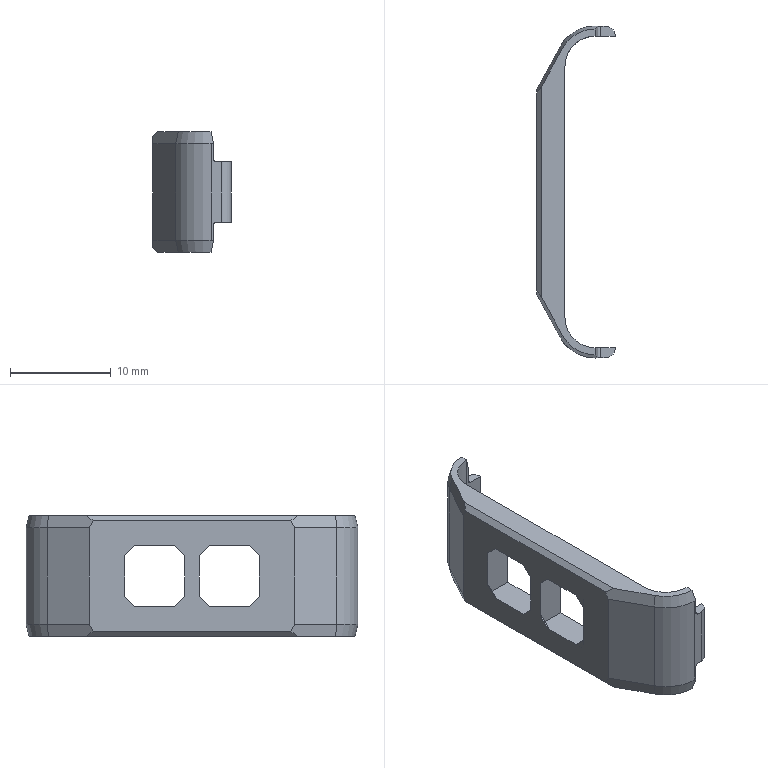Part | STEP file | [OP-85136]-6 | 1 solid | 66 faces | box 7.8 x 33 x 12 mm | volume 757.289 mm3 | plane 52 | cylinder 10 | cone 4 | commonest cylinder face diameters 0.6 x4 2 x2 6 x2 8 x2